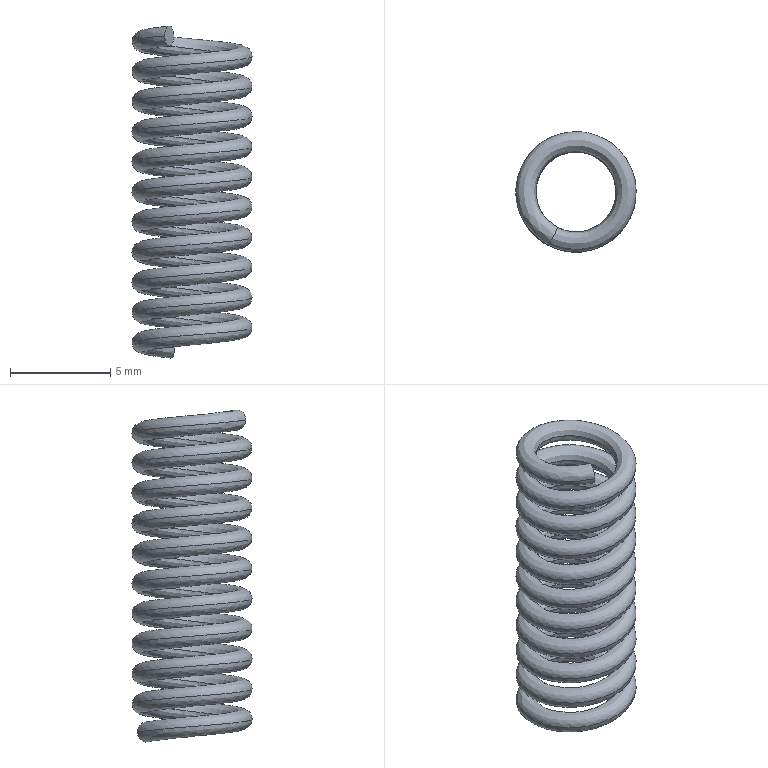Part | SolidWorks | features BaseBody 1 | 1 solid | 4 faces | box 5.993 x 5.996 x 16.531 mm | volume 125.487 mm3 | spline 2 | plane 2